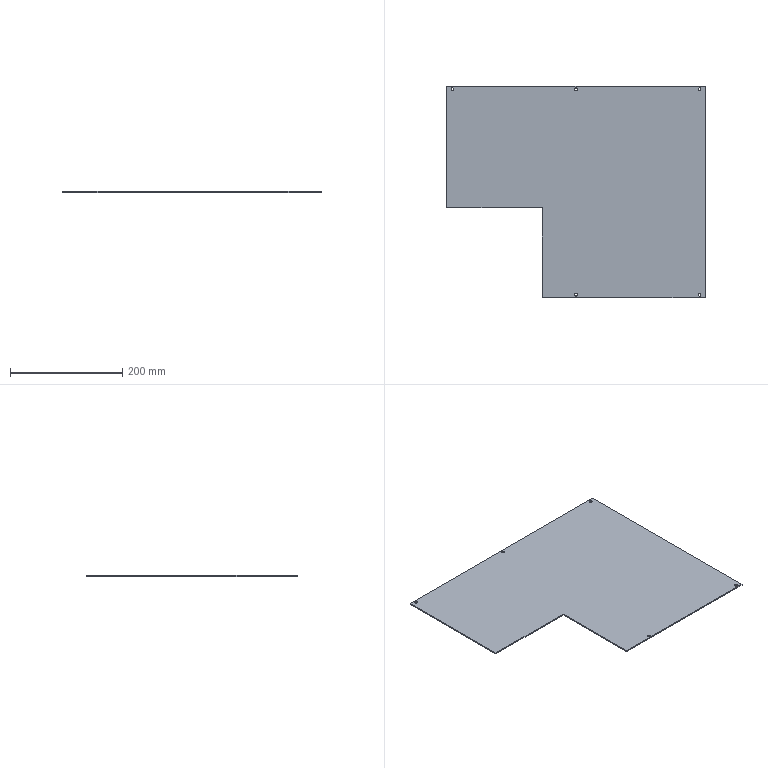Part | STEP file | Station three mount plate | 1 solid | 18 faces | box 460 x 376 x 2 mm | volume 291324 mm3 | cylinder 10 | plane 8 | commonest cylinder face diameters 5 x10
STEP:
#1=CARTESIAN_POINT('',(0.,0.,0.));
#2=DIRECTION('',(0.,0.,1.));
#3=DIRECTION('',(1.,0.,0.));
#4=AXIS2_PLACEMENT_3D('',#1,#2,#3);
#5=CARTESIAN_POINT('',(-217.5,183.,0.));
#6=VERTEX_POINT('',#5);
#7=CARTESIAN_POINT('',(-217.5,183.,2.));
#8=VERTEX_POINT('',#7);
#9=CARTESIAN_POINT('',(-217.5,183.,0.));
#10=DIRECTION('',(0.,0.,1.));
#11=VECTOR('',#10,1.);
#12=LINE('',#9,#11);
#13=CARTESIAN_POINT('',(-220.,183.,0.));
#14=DIRECTION('',(0.,0.,1.));
#15=DIRECTION('',(1.,0.,0.));
#16=AXIS2_PLACEMENT_3D('',#13,#14,#15);
#17=CYLINDRICAL_SURFACE('',#16,2.5);
#18=CARTESIAN_POINT('',(6.283,0.));
#19=DIRECTION('',(0.,1.));
#20=VECTOR('',#19,1.);
#21=LINE('',#18,#20);
#22=(GEOMETRIC_REPRESENTATION_CONTEXT(2)PARAMETRIC_REPRESENTATION_CONTEXT()REPRESENTATION_CONTEXT('',''));
#23=DEFINITIONAL_REPRESENTATION('',(#21),#22);
#24=PCURVE('',#17,#23);
#25=CARTESIAN_POINT('',(-220.,183.,0.));
#26=DIRECTION('',(0.,0.,1.));
#27=DIRECTION('',(1.,0.,0.));
#28=AXIS2_PLACEMENT_3D('',#25,#26,#27);
#29=CYLINDRICAL_SURFACE('',#28,2.5);
#30=CARTESIAN_POINT('',(0.,0.));
#31=DIRECTION('',(0.,1.));
#32=VECTOR('',#31,1.);
#33=LINE('',#30,#32);
#34=(GEOMETRIC_REPRESENTATION_CONTEXT(2)PARAMETRIC_REPRESENTATION_CONTEXT()REPRESENTATION_CONTEXT('',''));
#35=DEFINITIONAL_REPRESENTATION('',(#33),#34);
#36=PCURVE('',#29,#35);
#37=SURFACE_CURVE('',#12,(#24,#36),.PCURVE_S1.);
#38=EDGE_CURVE('',#6,#8,#37,.T.);
#39=ORIENTED_EDGE('',*,*,#38,.T.);
#40=CARTESIAN_POINT('',(-222.5,183.,2.));
#41=VERTEX_POINT('',#40);
#42=CARTESIAN_POINT('',(-220.,183.,2.));
#43=DIRECTION('',(0.,0.,-1.));
#44=DIRECTION('',(1.,0.,0.));
#45=AXIS2_PLACEMENT_3D('',#42,#43,#44);
#46=CIRCLE('',#45,2.5);
#47=CARTESIAN_POINT('',(6.283,2.));
#48=DIRECTION('',(-1.,0.));
#49=VECTOR('',#48,1.);
#50=LINE('',#47,#49);
#51=(GEOMETRIC_REPRESENTATION_CONTEXT(2)PARAMETRIC_REPRESENTATION_CONTEXT()REPRESENTATION_CONTEXT('',''));
#52=DEFINITIONAL_REPRESENTATION('',(#50),#51);
#53=PCURVE('',#17,#52);
#54=CARTESIAN_POINT('',(-230.,-188.,2.));
#55=DIRECTION('',(0.,0.,1.));
#56=DIRECTION('',(1.,0.,0.));
#57=AXIS2_PLACEMENT_3D('',#54,#55,#56);
#58=PLANE('',#57);
#59=CARTESIAN_POINT('',(12.5,371.));
#60=CARTESIAN_POINT('',(12.5,366.67));
#61=CARTESIAN_POINT('',(8.75,368.835));
#62=CARTESIAN_POINT('',(5.,371.));
#63=CARTESIAN_POINT('',(8.75,373.165));
#64=CARTESIAN_POINT('',(12.5,375.33));
#65=CARTESIAN_POINT('',(12.5,371.));
#66=(BOUNDED_CURVE()B_SPLINE_CURVE(2,(#59,#60,#61,#62,#63,#64,#65),.UNSPECIFIED.,.T.,.F.)B_SPLINE_CURVE_WITH_KNOTS((1,2,2,2,2,1),(-2.094,0.,2.094,4.189,6.283,8.378),.UNSPECIFIED.)CURVE()GEOMETRIC_REPRESENTATION_ITEM()RATIONAL_B_SPLINE_CURVE((1.,0.5,1.,0.5,1.,0.5,1.))REPRESENTATION_ITEM(''));
#67=(GEOMETRIC_REPRESENTATION_CONTEXT(2)PARAMETRIC_REPRESENTATION_CONTEXT()REPRESENTATION_CONTEXT('',''));
#68=DEFINITIONAL_REPRESENTATION('',(#66),#67);
#69=PCURVE('',#58,#68);
#70=SURFACE_CURVE('',#46,(#53,#69),.PCURVE_S1.);
#71=EDGE_CURVE('',#8,#41,#70,.T.);
#72=ORIENTED_EDGE('',*,*,#71,.T.);
#73=CARTESIAN_POINT('',(-222.5,183.,0.));
#74=VERTEX_POINT('',#73);
#75=CARTESIAN_POINT('',(-222.5,183.,0.));
#76=DIRECTION('',(0.,0.,1.));
#77=VECTOR('',#76,1.);
#78=LINE('',#75,#77);
#79=CARTESIAN_POINT('',(3.142,0.));
#80=DIRECTION('',(0.,1.));
#81=VECTOR('',#80,1.);
#82=LINE('',#79,#81);
#83=(GEOMETRIC_REPRESENTATION_CONTEXT(2)PARAMETRIC_REPRESENTATION_CONTEXT()REPRESENTATION_CONTEXT('',''));
#84=DEFINITIONAL_REPRESENTATION('',(#82),#83);
#85=PCURVE('',#17,#84);
#86=CARTESIAN_POINT('',(3.142,0.));
#87=DIRECTION('',(0.,1.));
#88=VECTOR('',#87,1.);
#89=LINE('',#86,#88);
#90=(GEOMETRIC_REPRESENTATION_CONTEXT(2)PARAMETRIC_REPRESENTATION_CONTEXT()REPRESENTATION_CONTEXT('',''));
#91=DEFINITIONAL_REPRESENTATION('',(#89),#90);
#92=PCURVE('',#29,#91);
#93=SURFACE_CURVE('',#78,(#85,#92),.PCURVE_S1.);
#94=EDGE_CURVE('',#74,#41,#93,.T.);
#95=ORIENTED_EDGE('',*,*,#94,.F.);
#96=CARTESIAN_POINT('',(-220.,183.,0.));
#97=DIRECTION('',(0.,0.,1.));
#98=DIRECTION('',(1.,0.,0.));
#99=AXIS2_PLACEMENT_3D('',#96,#97,#98);
#100=CIRCLE('',#99,2.5);
#101=CARTESIAN_POINT('',(0.,0.));
#102=DIRECTION('',(1.,0.));
#103=VECTOR('',#102,1.);
#104=LINE('',#101,#103);
#105=(GEOMETRIC_REPRESENTATION_CONTEXT(2)PARAMETRIC_REPRESENTATION_CONTEXT()REPRESENTATION_CONTEXT('',''));
#106=DEFINITIONAL_REPRESENTATION('',(#104),#105);
#107=PCURVE('',#17,#106);
#108=CARTESIAN_POINT('',(-230.,-188.,0.));
#109=DIRECTION('',(0.,0.,1.));
#110=DIRECTION('',(1.,0.,0.));
#111=AXIS2_PLACEMENT_3D('',#108,#109,#110);
#112=PLANE('',#111);
#113=CARTESIAN_POINT('',(10.,371.));
#114=DIRECTION('',(1.,0.));
#115=AXIS2_PLACEMENT_2D('',#113,#114);
#116=CIRCLE('',#115,2.5);
#117=(GEOMETRIC_REPRESENTATION_CONTEXT(2)PARAMETRIC_REPRESENTATION_CONTEXT()REPRESENTATION_CONTEXT('',''));
#118=DEFINITIONAL_REPRESENTATION('',(#116),#117);
#119=PCURVE('',#112,#118);
#120=SURFACE_CURVE('',#100,(#107,#119),.PCURVE_S1.);
#121=EDGE_CURVE('',#74,#6,#120,.T.);
#122=ORIENTED_EDGE('',*,*,#121,.T.);
#123=EDGE_LOOP('',(#39,#72,#95,#122));
#124=FACE_BOUND('',#123,.F.);
#125=ADVANCED_FACE('',(#124),#17,.F.);
#126=CARTESIAN_POINT('',(222.5,183.,0.));
#127=VERTEX_POINT('',#126);
#128=CARTESIAN_POINT('',(222.5,183.,2.));
#129=VERTEX_POINT('',#128);
#130=CARTESIAN_POINT('',(222.5,183.,0.));
#131=DIRECTION('',(0.,0.,1.));
#132=VECTOR('',#131,1.);
#133=LINE('',#130,#132);
#134=CARTESIAN_POINT('',(220.,183.,0.));
#135=DIRECTION('',(0.,0.,1.));
#136=DIRECTION('',(1.,0.,0.));
#137=AXIS2_PLACEMENT_3D('',#134,#135,#136);
#138=CYLINDRICAL_SURFACE('',#137,2.5);
#139=CARTESIAN_POINT('',(6.283,0.));
#140=DIRECTION('',(0.,1.));
#141=VECTOR('',#140,1.);
#142=LINE('',#139,#141);
#143=(GEOMETRIC_REPRESENTATION_CONTEXT(2)PARAMETRIC_REPRESENTATION_CONTEXT()REPRESENTATION_CONTEXT('',''));
#144=DEFINITIONAL_REPRESENTATION('',(#142),#143);
#145=PCURVE('',#138,#144);
#146=CARTESIAN_POINT('',(220.,183.,0.));
#147=DIRECTION('',(0.,0.,1.));
#148=DIRECTION('',(1.,0.,0.));
#149=AXIS2_PLACEMENT_3D('',#146,#147,#148);
#150=CYLINDRICAL_SURFACE('',#149,2.5);
#151=CARTESIAN_POINT('',(0.,0.));
#152=DIRECTION('',(0.,1.));
#153=VECTOR('',#152,1.);
#154=LINE('',#151,#153);
#155=(GEOMETRIC_REPRESENTATION_CONTEXT(2)PARAMETRIC_REPRESENTATION_CONTEXT()REPRESENTATION_CONTEXT('',''));
#156=DEFINITIONAL_REPRESENTATION('',(#154),#155);
#157=PCURVE('',#150,#156);
#158=SURFACE_CURVE('',#133,(#145,#157),.PCURVE_S1.);
#159=EDGE_CURVE('',#127,#129,#158,.T.);
#160=ORIENTED_EDGE('',*,*,#159,.T.);
#161=CARTESIAN_POINT('',(217.5,183.,2.));
#162=VERTEX_POINT('',#161);
#163=CARTESIAN_POINT('',(220.,183.,2.));
#164=DIRECTION('',(0.,0.,-1.));
#165=DIRECTION('',(1.,0.,0.));
#166=AXIS2_PLACEMENT_3D('',#163,#164,#165);
#167=CIRCLE('',#166,2.5);
#168=CARTESIAN_POINT('',(6.283,2.));
#169=DIRECTION('',(-1.,0.));
#170=VECTOR('',#169,1.);
#171=LINE('',#168,#170);
#172=(GEOMETRIC_REPRESENTATION_CONTEXT(2)PARAMETRIC_REPRESENTATION_CONTEXT()REPRESENTATION_CONTEXT('',''));
#173=DEFINITIONAL_REPRESENTATION('',(#171),#172);
#174=PCURVE('',#138,#173);
#175=CARTESIAN_POINT('',(452.5,371.));
#176=CARTESIAN_POINT('',(452.5,366.67));
#177=CARTESIAN_POINT('',(448.75,368.835));
#178=CARTESIAN_POINT('',(445.,371.));
#179=CARTESIAN_POINT('',(448.75,373.165));
#180=CARTESIAN_POINT('',(452.5,375.33));
#181=CARTESIAN_POINT('',(452.5,371.));
#182=(BOUNDED_CURVE()B_SPLINE_CURVE(2,(#175,#176,#177,#178,#179,#180,#181),.UNSPECIFIED.,.T.,.F.)B_SPLINE_CURVE_WITH_KNOTS((1,2,2,2,2,1),(-2.094,0.,2.094,4.189,6.283,8.378),.UNSPECIFIED.)CURVE()GEOMETRIC_REPRESENTATION_ITEM()RATIONAL_B_SPLINE_CURVE((1.,0.5,1.,0.5,1.,0.5,1.))REPRESENTATION_ITEM(''));
#183=(GEOMETRIC_REPRESENTATION_CONTEXT(2)PARAMETRIC_REPRESENTATION_CONTEXT()REPRESENTATION_CONTEXT('',''));
#184=DEFINITIONAL_REPRESENTATION('',(#182),#183);
#185=PCURVE('',#58,#184);
#186=SURFACE_CURVE('',#167,(#174,#185),.PCURVE_S1.);
#187=EDGE_CURVE('',#129,#162,#186,.T.);
#188=ORIENTED_EDGE('',*,*,#187,.T.);
#189=CARTESIAN_POINT('',(217.5,183.,0.));
#190=VERTEX_POINT('',#189);
#191=CARTESIAN_POINT('',(217.5,183.,0.));
#192=DIRECTION('',(0.,0.,1.));
#193=VECTOR('',#192,1.);
#194=LINE('',#191,#193);
#195=CARTESIAN_POINT('',(3.142,0.));
#196=DIRECTION('',(0.,1.));
#197=VECTOR('',#196,1.);
#198=LINE('',#195,#197);
#199=(GEOMETRIC_REPRESENTATION_CONTEXT(2)PARAMETRIC_REPRESENTATION_CONTEXT()REPRESENTATION_CONTEXT('',''));
#200=DEFINITIONAL_REPRESENTATION('',(#198),#199);
#201=PCURVE('',#138,#200);
#202=CARTESIAN_POINT('',(3.142,0.));
#203=DIRECTION('',(0.,1.));
#204=VECTOR('',#203,1.);
#205=LINE('',#202,#204);
#206=(GEOMETRIC_REPRESENTATION_CONTEXT(2)PARAMETRIC_REPRESENTATION_CONTEXT()REPRESENTATION_CONTEXT('',''));
#207=DEFINITIONAL_REPRESENTATION('',(#205),#206);
#208=PCURVE('',#150,#207);
#209=SURFACE_CURVE('',#194,(#201,#208),.PCURVE_S1.);
#210=EDGE_CURVE('',#190,#162,#209,.T.);
#211=ORIENTED_EDGE('',*,*,#210,.F.);
#212=CARTESIAN_POINT('',(220.,183.,0.));
#213=DIRECTION('',(0.,0.,1.));
#214=DIRECTION('',(1.,0.,0.));
#215=AXIS2_PLACEMENT_3D('',#212,#213,#214);
#216=CIRCLE('',#215,2.5);
#217=CARTESIAN_POINT('',(0.,0.));
#218=DIRECTION('',(1.,0.));
#219=VECTOR('',#218,1.);
#220=LINE('',#217,#219);
#221=(GEOMETRIC_REPRESENTATION_CONTEXT(2)PARAMETRIC_REPRESENTATION_CONTEXT()REPRESENTATION_CONTEXT('',''));
#222=DEFINITIONAL_REPRESENTATION('',(#220),#221);
#223=PCURVE('',#138,#222);
#224=CARTESIAN_POINT('',(450.,371.));
#225=DIRECTION('',(1.,0.));
#226=AXIS2_PLACEMENT_2D('',#224,#225);
#227=CIRCLE('',#226,2.5);
#228=(GEOMETRIC_REPRESENTATION_CONTEXT(2)PARAMETRIC_REPRESENTATION_CONTEXT()REPRESENTATION_CONTEXT('',''));
#229=DEFINITIONAL_REPRESENTATION('',(#227),#228);
#230=PCURVE('',#112,#229);
#231=SURFACE_CURVE('',#216,(#223,#230),.PCURVE_S1.);
#232=EDGE_CURVE('',#190,#127,#231,.T.);
#233=ORIENTED_EDGE('',*,*,#232,.T.);
#234=EDGE_LOOP('',(#160,#188,#211,#233));
#235=FACE_BOUND('',#234,.F.);
#236=ADVANCED_FACE('',(#235),#138,.F.);
#237=CARTESIAN_POINT('',(2.5,-183.,0.));
#238=VERTEX_POINT('',#237);
#239=CARTESIAN_POINT('',(2.5,-183.,2.));
#240=VERTEX_POINT('',#239);
#241=CARTESIAN_POINT('',(2.5,-183.,0.));
#242=DIRECTION('',(0.,0.,1.));
#243=VECTOR('',#242,1.);
#244=LINE('',#241,#243);
#245=CARTESIAN_POINT('',(0.,-183.,0.));
#246=DIRECTION('',(0.,0.,1.));
#247=DIRECTION('',(1.,0.,0.));
#248=AXIS2_PLACEMENT_3D('',#245,#246,#247);
#249=CYLINDRICAL_SURFACE('',#248,2.5);
#250=CARTESIAN_POINT('',(6.283,0.));
#251=DIRECTION('',(0.,1.));
#252=VECTOR('',#251,1.);
#253=LINE('',#250,#252);
#254=(GEOMETRIC_REPRESENTATION_CONTEXT(2)PARAMETRIC_REPRESENTATION_CONTEXT()REPRESENTATION_CONTEXT('',''));
#255=DEFINITIONAL_REPRESENTATION('',(#253),#254);
#256=PCURVE('',#249,#255);
#257=CARTESIAN_POINT('',(0.,-183.,0.));
#258=DIRECTION('',(0.,0.,1.));
#259=DIRECTION('',(1.,0.,0.));
#260=AXIS2_PLACEMENT_3D('',#257,#258,#259);
#261=CYLINDRICAL_SURFACE('',#260,2.5);
#262=CARTESIAN_POINT('',(0.,0.));
#263=DIRECTION('',(0.,1.));
#264=VECTOR('',#263,1.);
#265=LINE('',#262,#264);
#266=(GEOMETRIC_REPRESENTATION_CONTEXT(2)PARAMETRIC_REPRESENTATION_CONTEXT()REPRESENTATION_CONTEXT('',''));
#267=DEFINITIONAL_REPRESENTATION('',(#265),#266);
#268=PCURVE('',#261,#267);
#269=SURFACE_CURVE('',#244,(#256,#268),.PCURVE_S1.);
#270=EDGE_CURVE('',#238,#240,#269,.T.);
#271=ORIENTED_EDGE('',*,*,#270,.T.);
#272=CARTESIAN_POINT('',(-2.5,-183.,2.));
#273=VERTEX_POINT('',#272);
#274=CARTESIAN_POINT('',(0.,-183.,2.));
#275=DIRECTION('',(0.,0.,-1.));
#276=DIRECTION('',(1.,0.,0.));
#277=AXIS2_PLACEMENT_3D('',#274,#275,#276);
#278=CIRCLE('',#277,2.5);
#279=CARTESIAN_POINT('',(6.283,2.));
#280=DIRECTION('',(-1.,0.));
#281=VECTOR('',#280,1.);
#282=LINE('',#279,#281);
#283=(GEOMETRIC_REPRESENTATION_CONTEXT(2)PARAMETRIC_REPRESENTATION_CONTEXT()REPRESENTATION_CONTEXT('',''));
#284=DEFINITIONAL_REPRESENTATION('',(#282),#283);
#285=PCURVE('',#249,#284);
#286=CARTESIAN_POINT('',(232.5,5.));
#287=CARTESIAN_POINT('',(232.5,0.6699));
#288=CARTESIAN_POINT('',(228.75,2.835));
#289=CARTESIAN_POINT('',(225.,5.));
#290=CARTESIAN_POINT('',(228.75,7.165));
#291=CARTESIAN_POINT('',(232.5,9.33));
#292=CARTESIAN_POINT('',(232.5,5.));
#293=(BOUNDED_CURVE()B_SPLINE_CURVE(2,(#286,#287,#288,#289,#290,#291,#292),.UNSPECIFIED.,.T.,.F.)B_SPLINE_CURVE_WITH_KNOTS((1,2,2,2,2,1),(-2.094,0.,2.094,4.189,6.283,8.378),.UNSPECIFIED.)CURVE()GEOMETRIC_REPRESENTATION_ITEM()RATIONAL_B_SPLINE_CURVE((1.,0.5,1.,0.5,1.,0.5,1.))REPRESENTATION_ITEM(''));
#294=(GEOMETRIC_REPRESENTATION_CONTEXT(2)PARAMETRIC_REPRESENTATION_CONTEXT()REPRESENTATION_CONTEXT('',''));
#295=DEFINITIONAL_REPRESENTATION('',(#293),#294);
#296=PCURVE('',#58,#295);
#297=SURFACE_CURVE('',#278,(#285,#296),.PCURVE_S1.);
#298=EDGE_CURVE('',#240,#273,#297,.T.);
#299=ORIENTED_EDGE('',*,*,#298,.T.);
#300=CARTESIAN_POINT('',(-2.5,-183.,0.));
#301=VERTEX_POINT('',#300);
#302=CARTESIAN_POINT('',(-2.5,-183.,0.));
#303=DIRECTION('',(0.,0.,1.));
#304=VECTOR('',#303,1.);
#305=LINE('',#302,#304);
#306=CARTESIAN_POINT('',(3.142,0.));
#307=DIRECTION('',(0.,1.));
#308=VECTOR('',#307,1.);
#309=LINE('',#306,#308);
#310=(GEOMETRIC_REPRESENTATION_CONTEXT(2)PARAMETRIC_REPRESENTATION_CONTEXT()REPRESENTATION_CONTEXT('',''));
#311=DEFINITIONAL_REPRESENTATION('',(#309),#310);
#312=PCURVE('',#249,#311);
#313=CARTESIAN_POINT('',(3.142,0.));
#314=DIRECTION('',(0.,1.));
#315=VECTOR('',#314,1.);
#316=LINE('',#313,#315);
#317=(GEOMETRIC_REPRESENTATION_CONTEXT(2)PARAMETRIC_REPRESENTATION_CONTEXT()REPRESENTATION_CONTEXT('',''));
#318=DEFINITIONAL_REPRESENTATION('',(#316),#317);
#319=PCURVE('',#261,#318);
#320=SURFACE_CURVE('',#305,(#312,#319),.PCURVE_S1.);
#321=EDGE_CURVE('',#301,#273,#320,.T.);
#322=ORIENTED_EDGE('',*,*,#321,.F.);
#323=CARTESIAN_POINT('',(0.,-183.,0.));
#324=DIRECTION('',(0.,0.,1.));
#325=DIRECTION('',(1.,0.,0.));
#326=AXIS2_PLACEMENT_3D('',#323,#324,#325);
#327=CIRCLE('',#326,2.5);
#328=CARTESIAN_POINT('',(0.,0.));
#329=DIRECTION('',(1.,0.));
#330=VECTOR('',#329,1.);
#331=LINE('',#328,#330);
#332=(GEOMETRIC_REPRESENTATION_CONTEXT(2)PARAMETRIC_REPRESENTATION_CONTEXT()REPRESENTATION_CONTEXT('',''));
#333=DEFINITIONAL_REPRESENTATION('',(#331),#332);
#334=PCURVE('',#249,#333);
#335=CARTESIAN_POINT('',(230.,5.));
#336=DIRECTION('',(1.,0.));
#337=AXIS2_PLACEMENT_2D('',#335,#336);
#338=CIRCLE('',#337,2.5);
#339=(GEOMETRIC_REPRESENTATION_CONTEXT(2)PARAMETRIC_REPRESENTATION_CONTEXT()REPRESENTATION_CONTEXT('',''));
#340=DEFINITIONAL_REPRESENTATION('',(#338),#339);
#341=PCURVE('',#112,#340);
#342=SURFACE_CURVE('',#327,(#334,#341),.PCURVE_S1.);
#343=EDGE_CURVE('',#301,#238,#342,.T.);
#344=ORIENTED_EDGE('',*,*,#343,.T.);
#345=EDGE_LOOP('',(#271,#299,#322,#344));
#346=FACE_BOUND('',#345,.F.);
#347=ADVANCED_FACE('',(#346),#249,.F.);
#348=CARTESIAN_POINT('',(222.5,-183.,0.));
#349=VERTEX_POINT('',#348);
#350=CARTESIAN_POINT('',(222.5,-183.,2.));
#351=VERTEX_POINT('',#350);
#352=CARTESIAN_POINT('',(222.5,-183.,0.));
#353=DIRECTION('',(0.,0.,1.));
#354=VECTOR('',#353,1.);
#355=LINE('',#352,#354);
#356=CARTESIAN_POINT('',(220.,-183.,0.));
#357=DIRECTION('',(0.,0.,1.));
#358=DIRECTION('',(1.,0.,0.));
#359=AXIS2_PLACEMENT_3D('',#356,#357,#358);
#360=CYLINDRICAL_SURFACE('',#359,2.5);
#361=CARTESIAN_POINT('',(6.283,0.));
#362=DIRECTION('',(0.,1.));
#363=VECTOR('',#362,1.);
#364=LINE('',#361,#363);
#365=(GEOMETRIC_REPRESENTATION_CONTEXT(2)PARAMETRIC_REPRESENTATION_CONTEXT()REPRESENTATION_CONTEXT('',''));
#366=DEFINITIONAL_REPRESENTATION('',(#364),#365);
#367=PCURVE('',#360,#366);
#368=CARTESIAN_POINT('',(220.,-183.,0.));
#369=DIRECTION('',(0.,0.,1.));
#370=DIRECTION('',(1.,0.,0.));
#371=AXIS2_PLACEMENT_3D('',#368,#369,#370);
#372=CYLINDRICAL_SURFACE('',#371,2.5);
#373=CARTESIAN_POINT('',(0.,0.));
#374=DIRECTION('',(0.,1.));
#375=VECTOR('',#374,1.);
#376=LINE('',#373,#375);
#377=(GEOMETRIC_REPRESENTATION_CONTEXT(2)PARAMETRIC_REPRESENTATION_CONTEXT()REPRESENTATION_CONTEXT('',''));
#378=DEFINITIONAL_REPRESENTATION('',(#376),#377);
#379=PCURVE('',#372,#378);
#380=SURFACE_CURVE('',#355,(#367,#379),.PCURVE_S1.);
#381=EDGE_CURVE('',#349,#351,#380,.T.);
#382=ORIENTED_EDGE('',*,*,#381,.T.);
#383=CARTESIAN_POINT('',(217.5,-183.,2.));
#384=VERTEX_POINT('',#383);
#385=CARTESIAN_POINT('',(220.,-183.,2.));
#386=DIRECTION('',(0.,0.,-1.));
#387=DIRECTION('',(1.,0.,0.));
#388=AXIS2_PLACEMENT_3D('',#385,#386,#387);
#389=CIRCLE('',#388,2.5);
#390=CARTESIAN_POINT('',(6.283,2.));
#391=DIRECTION('',(-1.,0.));
#392=VECTOR('',#391,1.);
#393=LINE('',#390,#392);
#394=(GEOMETRIC_REPRESENTATION_CONTEXT(2)PARAMETRIC_REPRESENTATION_CONTEXT()REPRESENTATION_CONTEXT('',''));
#395=DEFINITIONAL_REPRESENTATION('',(#393),#394);
#396=PCURVE('',#360,#395);
#397=CARTESIAN_POINT('',(452.5,5.));
#398=CARTESIAN_POINT('',(452.5,0.6699));
#399=CARTESIAN_POINT('',(448.75,2.835));
#400=CARTESIAN_POINT('',(445.,5.));
#401=CARTESIAN_POINT('',(448.75,7.165));
#402=CARTESIAN_POINT('',(452.5,9.33));
#403=CARTESIAN_POINT('',(452.5,5.));
#404=(BOUNDED_CURVE()B_SPLINE_CURVE(2,(#397,#398,#399,#400,#401,#402,#403),.UNSPECIFIED.,.T.,.F.)B_SPLINE_CURVE_WITH_KNOTS((1,2,2,2,2,1),(-2.094,0.,2.094,4.189,6.283,8.378),.UNSPECIFIED.)CURVE()GEOMETRIC_REPRESENTATION_ITEM()RATIONAL_B_SPLINE_CURVE((1.,0.5,1.,0.5,1.,0.5,1.))REPRESENTATION_ITEM(''));
#405=(GEOMETRIC_REPRESENTATION_CONTEXT(2)PARAMETRIC_REPRESENTATION_CONTEXT()REPRESENTATION_CONTEXT('',''));
#406=DEFINITIONAL_REPRESENTATION('',(#404),#405);
#407=PCURVE('',#58,#406);
#408=SURFACE_CURVE('',#389,(#396,#407),.PCURVE_S1.);
#409=EDGE_CURVE('',#351,#384,#408,.T.);
#410=ORIENTED_EDGE('',*,*,#409,.T.);
#411=CARTESIAN_POINT('',(217.5,-183.,0.));
#412=VERTEX_POINT('',#411);
#413=CARTESIAN_POINT('',(217.5,-183.,0.));
#414=DIRECTION('',(0.,0.,1.));
#415=VECTOR('',#414,1.);
#416=LINE('',#413,#415);
#417=CARTESIAN_POINT('',(3.142,0.));
#418=DIRECTION('',(0.,1.));
#419=VECTOR('',#418,1.);
#420=LINE('',#417,#419);
#421=(GEOMETRIC_REPRESENTATION_CONTEXT(2)PARAMETRIC_REPRESENTATION_CONTEXT()REPRESENTATION_CONTEXT('',''));
#422=DEFINITIONAL_REPRESENTATION('',(#420),#421);
#423=PCURVE('',#360,#422);
#424=CARTESIAN_POINT('',(3.142,0.));
#425=DIRECTION('',(0.,1.));
#426=VECTOR('',#425,1.);
#427=LINE('',#424,#426);
#428=(GEOMETRIC_REPRESENTATION_CONTEXT(2)PARAMETRIC_REPRESENTATION_CONTEXT()REPRESENTATION_CONTEXT('',''));
#429=DEFINITIONAL_REPRESENTATION('',(#427),#428);
#430=PCURVE('',#372,#429);
#431=SURFACE_CURVE('',#416,(#423,#430),.PCURVE_S1.);
#432=EDGE_CURVE('',#412,#384,#431,.T.);
#433=ORIENTED_EDGE('',*,*,#432,.F.);
#434=CARTESIAN_POINT('',(220.,-183.,0.));
#435=DIRECTION('',(0.,0.,1.));
#436=DIRECTION('',(1.,0.,0.));
#437=AXIS2_PLACEMENT_3D('',#434,#435,#436);
#438=CIRCLE('',#437,2.5);
#439=CARTESIAN_POINT('',(0.,0.));
#440=DIRECTION('',(1.,0.));
#441=VECTOR('',#440,1.);
#442=LINE('',#439,#441);
#443=(GEOMETRIC_REPRESENTATION_CONTEXT(2)PARAMETRIC_REPRESENTATION_CONTEXT()REPRESENTATION_CONTEXT('',''));
#444=DEFINITIONAL_REPRESENTATION('',(#442),#443);
#445=PCURVE('',#360,#444);
#446=CARTESIAN_POINT('',(450.,5.));
#447=DIRECTION('',(1.,0.));
#448=AXIS2_PLACEMENT_2D('',#446,#447);
#449=CIRCLE('',#448,2.5);
#450=(GEOMETRIC_REPRESENTATION_CONTEXT(2)PARAMETRIC_REPRESENTATION_CONTEXT()REPRESENTATION_CONTEXT('',''));
#451=DEFINITIONAL_REPRESENTATION('',(#449),#450);
#452=PCURVE('',#112,#451);
#453=SURFACE_CURVE('',#438,(#445,#452),.PCURVE_S1.);
#454=EDGE_CURVE('',#412,#349,#453,.T.);
#455=ORIENTED_EDGE('',*,*,#454,.T.);
#456=EDGE_LOOP('',(#382,#410,#433,#455));
#457=FACE_BOUND('',#456,.F.);
#458=ADVANCED_FACE('',(#457),#360,.F.);
#459=CARTESIAN_POINT('',(2.5,183.,0.));
#460=VERTEX_POINT('',#459);
#461=CARTESIAN_POINT('',(2.5,183.,2.));
#462=VERTEX_POINT('',#461);
#463=CARTESIAN_POINT('',(2.5,183.,0.));
#464=DIRECTION('',(0.,0.,1.));
#465=VECTOR('',#464,1.);
#466=LINE('',#463,#465);
#467=CARTESIAN_POINT('',(0.,183.,0.));
#468=DIRECTION('',(0.,0.,1.));
#469=DIRECTION('',(1.,0.,0.));
#470=AXIS2_PLACEMENT_3D('',#467,#468,#469);
#471=CYLINDRICAL_SURFACE('',#470,2.5);
#472=CARTESIAN_POINT('',(6.283,0.));
#473=DIRECTION('',(0.,1.));
#474=VECTOR('',#473,1.);
#475=LINE('',#472,#474);
#476=(GEOMETRIC_REPRESENTATION_CONTEXT(2)PARAMETRIC_REPRESENTATION_CONTEXT()REPRESENTATION_CONTEXT('',''));
#477=DEFINITIONAL_REPRESENTATION('',(#475),#476);
#478=PCURVE('',#471,#477);
#479=CARTESIAN_POINT('',(0.,183.,0.));
#480=DIRECTION('',(0.,0.,1.));
#481=DIRECTION('',(1.,0.,0.));
#482=AXIS2_PLACEMENT_3D('',#479,#480,#481);
#483=CYLINDRICAL_SURFACE('',#482,2.5);
#484=CARTESIAN_POINT('',(0.,0.));
#485=DIRECTION('',(0.,1.));
#486=VECTOR('',#485,1.);
#487=LINE('',#484,#486);
#488=(GEOMETRIC_REPRESENTATION_CONTEXT(2)PARAMETRIC_REPRESENTATION_CONTEXT()REPRESENTATION_CONTEXT('',''));
#489=DEFINITIONAL_REPRESENTATION('',(#487),#488);
#490=PCURVE('',#483,#489);
#491=SURFACE_CURVE('',#466,(#478,#490),.PCURVE_S1.);
#492=EDGE_CURVE('',#460,#462,#491,.T.);
#493=ORIENTED_EDGE('',*,*,#492,.T.);
#494=CARTESIAN_POINT('',(-2.5,183.,2.));
#495=VERTEX_POINT('',#494);
#496=CARTESIAN_POINT('',(0.,183.,2.));
#497=DIRECTION('',(0.,0.,-1.));
#498=DIRECTION('',(1.,0.,0.));
#499=AXIS2_PLACEMENT_3D('',#496,#497,#498);
#500=CIRCLE('',#499,2.5);
#501=CARTESIAN_POINT('',(6.283,2.));
#502=DIRECTION('',(-1.,0.));
#503=VECTOR('',#502,1.);
#504=LINE('',#501,#503);
#505=(GEOMETRIC_REPRESENTATION_CONTEXT(2)PARAMETRIC_REPRESENTATION_CONTEXT()REPRESENTATION_CONTEXT('',''));
#506=DEFINITIONAL_REPRESENTATION('',(#504),#505);
#507=PCURVE('',#471,#506);
#508=CARTESIAN_POINT('',(232.5,371.));
#509=CARTESIAN_POINT('',(232.5,366.67));
#510=CARTESIAN_POINT('',(228.75,368.835));
#511=CARTESIAN_POINT('',(225.,371.));
#512=CARTESIAN_POINT('',(228.75,373.165));
#513=CARTESIAN_POINT('',(232.5,375.33));
#514=CARTESIAN_POINT('',(232.5,371.));
#515=(BOUNDED_CURVE()B_SPLINE_CURVE(2,(#508,#509,#510,#511,#512,#513,#514),.UNSPECIFIED.,.T.,.F.)B_SPLINE_CURVE_WITH_KNOTS((1,2,2,2,2,1),(-2.094,0.,2.094,4.189,6.283,8.378),.UNSPECIFIED.)CURVE()GEOMETRIC_REPRESENTATION_ITEM()RATIONAL_B_SPLINE_CURVE((1.,0.5,1.,0.5,1.,0.5,1.))REPRESENTATION_ITEM(''));
#516=(GEOMETRIC_REPRESENTATION_CONTEXT(2)PARAMETRIC_REPRESENTATION_CONTEXT()REPRESENTATION_CONTEXT('',''));
#517=DEFINITIONAL_REPRESENTATION('',(#515),#516);
#518=PCURVE('',#58,#517);
#519=SURFACE_CURVE('',#500,(#507,#518),.PCURVE_S1.);
#520=EDGE_CURVE('',#462,#495,#519,.T.);
#521=ORIENTED_EDGE('',*,*,#520,.T.);
#522=CARTESIAN_POINT('',(-2.5,183.,0.));
#523=VERTEX_POINT('',#522);
#524=CARTESIAN_POINT('',(-2.5,183.,0.));
#525=DIRECTION('',(0.,0.,1.));
#526=VECTOR('',#525,1.);
#527=LINE('',#524,#526);
#528=CARTESIAN_POINT('',(3.142,0.));
#529=DIRECTION('',(0.,1.));
#530=VECTOR('',#529,1.);
#531=LINE('',#528,#530);
#532=(GEOMETRIC_REPRESENTATION_CONTEXT(2)PARAMETRIC_REPRESENTATION_CONTEXT()REPRESENTATION_CONTEXT('',''));
#533=DEFINITIONAL_REPRESENTATION('',(#531),#532);
#534=PCURVE('',#471,#533);
#535=CARTESIAN_POINT('',(3.142,0.));
#536=DIRECTION('',(0.,1.));
#537=VECTOR('',#536,1.);
#538=LINE('',#535,#537);
#539=(GEOMETRIC_REPRESENTATION_CONTEXT(2)PARAMETRIC_REPRESENTATION_CONTEXT()REPRESENTATION_CONTEXT('',''));
#540=DEFINITIONAL_REPRESENTATION('',(#538),#539);
#541=PCURVE('',#483,#540);
#542=SURFACE_CURVE('',#527,(#534,#541),.PCURVE_S1.);
#543=EDGE_CURVE('',#523,#495,#542,.T.);
#544=ORIENTED_EDGE('',*,*,#543,.F.);
#545=CARTESIAN_POINT('',(0.,183.,0.));
#546=DIRECTION('',(0.,0.,1.));
#547=DIRECTION('',(1.,0.,0.));
#548=AXIS2_PLACEMENT_3D('',#545,#546,#547);
#549=CIRCLE('',#548,2.5);
#550=CARTESIAN_POINT('',(0.,0.));
#551=DIRECTION('',(1.,0.));
#552=VECTOR('',#551,1.);
#553=LINE('',#550,#552);
#554=(GEOMETRIC_REPRESENTATION_CONTEXT(2)PARAMETRIC_REPRESENTATION_CONTEXT()REPRESENTATION_CONTEXT('',''));
#555=DEFINITIONAL_REPRESENTATION('',(#553),#554);
#556=PCURVE('',#471,#555);
#557=CARTESIAN_POINT('',(230.,371.));
#558=DIRECTION('',(1.,0.));
#559=AXIS2_PLACEMENT_2D('',#557,#558);
#560=CIRCLE('',#559,2.5);
#561=(GEOMETRIC_REPRESENTATION_CONTEXT(2)PARAMETRIC_REPRESENTATION_CONTEXT()REPRESENTATION_CONTEXT('',''));
#562=DEFINITIONAL_REPRESENTATION('',(#560),#561);
#563=PCURVE('',#112,#562);
#564=SURFACE_CURVE('',#549,(#556,#563),.PCURVE_S1.);
#565=EDGE_CURVE('',#523,#460,#564,.T.);
#566=ORIENTED_EDGE('',*,*,#565,.T.);
#567=EDGE_LOOP('',(#493,#521,#544,#566));
#568=FACE_BOUND('',#567,.F.);
#569=ADVANCED_FACE('',(#568),#471,.F.);
#570=ORIENTED_EDGE('',*,*,#71,.T.);
#571=CARTESIAN_POINT('',(-220.,183.,2.));
#572=DIRECTION('',(0.,0.,-1.));
#573=DIRECTION('',(1.,0.,0.));
#574=AXIS2_PLACEMENT_3D('',#571,#572,#573);
#575=CIRCLE('',#574,2.5);
#576=CARTESIAN_POINT('',(12.5,371.));
#577=CARTESIAN_POINT('',(12.5,366.67));
#578=CARTESIAN_POINT('',(8.75,368.835));
#579=CARTESIAN_POINT('',(5.,371.));
#580=CARTESIAN_POINT('',(8.75,373.165));
#581=CARTESIAN_POINT('',(12.5,375.33));
#582=CARTESIAN_POINT('',(12.5,371.));
#583=(BOUNDED_CURVE()B_SPLINE_CURVE(2,(#576,#577,#578,#579,#580,#581,#582),.UNSPECIFIED.,.T.,.F.)B_SPLINE_CURVE_WITH_KNOTS((1,2,2,2,2,1),(-2.094,0.,2.094,4.189,6.283,8.378),.UNSPECIFIED.)CURVE()GEOMETRIC_REPRESENTATION_ITEM()RATIONAL_B_SPLINE_CURVE((1.,0.5,1.,0.5,1.,0.5,1.))REPRESENTATION_ITEM(''));
#584=(GEOMETRIC_REPRESENTATION_CONTEXT(2)PARAMETRIC_REPRESENTATION_CONTEXT()REPRESENTATION_CONTEXT('',''));
#585=DEFINITIONAL_REPRESENTATION('',(#583),#584);
#586=PCURVE('',#58,#585);
#587=CARTESIAN_POINT('',(6.283,2.));
#588=DIRECTION('',(-1.,0.));
#589=VECTOR('',#588,1.);
#590=LINE('',#587,#589);
#591=(GEOMETRIC_REPRESENTATION_CONTEXT(2)PARAMETRIC_REPRESENTATION_CONTEXT()REPRESENTATION_CONTEXT('',''));
#592=DEFINITIONAL_REPRESENTATION('',(#590),#591);
#593=PCURVE('',#29,#592);
#594=SURFACE_CURVE('',#575,(#586,#593),.PCURVE_S1.);
#595=EDGE_CURVE('',#41,#8,#594,.T.);
#596=ORIENTED_EDGE('',*,*,#595,.T.);
#597=EDGE_LOOP('',(#570,#596));
#598=FACE_BOUND('',#597,.T.);
#599=ORIENTED_EDGE('',*,*,#187,.T.);
#600=CARTESIAN_POINT('',(220.,183.,2.));
#601=DIRECTION('',(0.,0.,-1.));
#602=DIRECTION('',(1.,0.,0.));
#603=AXIS2_PLACEMENT_3D('',#600,#601,#602);
#604=CIRCLE('',#603,2.5);
#605=CARTESIAN_POINT('',(452.5,371.));
#606=CARTESIAN_POINT('',(452.5,366.67));
#607=CARTESIAN_POINT('',(448.75,368.835));
#608=CARTESIAN_POINT('',(445.,371.));
#609=CARTESIAN_POINT('',(448.75,373.165));
#610=CARTESIAN_POINT('',(452.5,375.33));
#611=CARTESIAN_POINT('',(452.5,371.));
#612=(BOUNDED_CURVE()B_SPLINE_CURVE(2,(#605,#606,#607,#608,#609,#610,#611),.UNSPECIFIED.,.T.,.F.)B_SPLINE_CURVE_WITH_KNOTS((1,2,2,2,2,1),(-2.094,0.,2.094,4.189,6.283,8.378),.UNSPECIFIED.)CURVE()GEOMETRIC_REPRESENTATION_ITEM()RATIONAL_B_SPLINE_CURVE((1.,0.5,1.,0.5,1.,0.5,1.))REPRESENTATION_ITEM(''));
#613=(GEOMETRIC_REPRESENTATION_CONTEXT(2)PARAMETRIC_REPRESENTATION_CONTEXT()REPRESENTATION_CONTEXT('',''));
#614=DEFINITIONAL_REPRESENTATION('',(#612),#613);
#615=PCURVE('',#58,#614);
#616=CARTESIAN_POINT('',(6.283,2.));
#617=DIRECTION('',(-1.,0.));
#618=VECTOR('',#617,1.);
#619=LINE('',#616,#618);
#620=(GEOMETRIC_REPRESENTATION_CONTEXT(2)PARAMETRIC_REPRESENTATION_CONTEXT()REPRESENTATION_CONTEXT('',''));
#621=DEFINITIONAL_REPRESENTATION('',(#619),#620);
#622=PCURVE('',#150,#621);
#623=SURFACE_CURVE('',#604,(#615,#622),.PCURVE_S1.);
#624=EDGE_CURVE('',#162,#129,#623,.T.);
#625=ORIENTED_EDGE('',*,*,#624,.T.);
#626=EDGE_LOOP('',(#599,#625));
#627=FACE_BOUND('',#626,.T.);
#628=ORIENTED_EDGE('',*,*,#298,.T.);
#629=CARTESIAN_POINT('',(0.,-183.,2.));
#630=DIRECTION('',(0.,0.,-1.));
#631=DIRECTION('',(1.,0.,0.));
#632=AXIS2_PLACEMENT_3D('',#629,#630,#631);
#633=CIRCLE('',#632,2.5);
#634=CARTESIAN_POINT('',(232.5,5.));
#635=CARTESIAN_POINT('',(232.5,0.6699));
#636=CARTESIAN_POINT('',(228.75,2.835));
#637=CARTESIAN_POINT('',(225.,5.));
#638=CARTESIAN_POINT('',(228.75,7.165));
#639=CARTESIAN_POINT('',(232.5,9.33));
#640=CARTESIAN_POINT('',(232.5,5.));
#641=(BOUNDED_CURVE()B_SPLINE_CURVE(2,(#634,#635,#636,#637,#638,#639,#640),.UNSPECIFIED.,.T.,.F.)B_SPLINE_CURVE_WITH_KNOTS((1,2,2,2,2,1),(-2.094,0.,2.094,4.189,6.283,8.378),.UNSPECIFIED.)CURVE()GEOMETRIC_REPRESENTATION_ITEM()RATIONAL_B_SPLINE_CURVE((1.,0.5,1.,0.5,1.,0.5,1.))REPRESENTATION_ITEM(''));
#642=(GEOMETRIC_REPRESENTATION_CONTEXT(2)PARAMETRIC_REPRESENTATION_CONTEXT()REPRESENTATION_CONTEXT('',''));
#643=DEFINITIONAL_REPRESENTATION('',(#641),#642);
#644=PCURVE('',#58,#643);
#645=CARTESIAN_POINT('',(6.283,2.));
#646=DIRECTION('',(-1.,0.));
#647=VECTOR('',#646,1.);
#648=LINE('',#645,#647);
#649=(GEOMETRIC_REPRESENTATION_CONTEXT(2)PARAMETRIC_REPRESENTATION_CONTEXT()REPRESENTATION_CONTEXT('',''));
#650=DEFINITIONAL_REPRESENTATION('',(#648),#649);
#651=PCURVE('',#261,#650);
#652=SURFACE_CURVE('',#633,(#644,#651),.PCURVE_S1.);
#653=EDGE_CURVE('',#273,#240,#652,.T.);
#654=ORIENTED_EDGE('',*,*,#653,.T.);
#655=EDGE_LOOP('',(#628,#654));
#656=FACE_BOUND('',#655,.T.);
#657=ORIENTED_EDGE('',*,*,#409,.T.);
#658=CARTESIAN_POINT('',(220.,-183.,2.));
#659=DIRECTION('',(0.,0.,-1.));
#660=DIRECTION('',(1.,0.,0.));
#661=AXIS2_PLACEMENT_3D('',#658,#659,#660);
#662=CIRCLE('',#661,2.5);
#663=CARTESIAN_POINT('',(452.5,5.));
#664=CARTESIAN_POINT('',(452.5,0.6699));
#665=CARTESIAN_POINT('',(448.75,2.835));
#666=CARTESIAN_POINT('',(445.,5.));
#667=CARTESIAN_POINT('',(448.75,7.165));
#668=CARTESIAN_POINT('',(452.5,9.33));
#669=CARTESIAN_POINT('',(452.5,5.));
#670=(BOUNDED_CURVE()B_SPLINE_CURVE(2,(#663,#664,#665,#666,#667,#668,#669),.UNSPECIFIED.,.T.,.F.)B_SPLINE_CURVE_WITH_KNOTS((1,2,2,2,2,1),(-2.094,0.,2.094,4.189,6.283,8.378),.UNSPECIFIED.)CURVE()GEOMETRIC_REPRESENTATION_ITEM()RATIONAL_B_SPLINE_CURVE((1.,0.5,1.,0.5,1.,0.5,1.))REPRESENTATION_ITEM(''));
#671=(GEOMETRIC_REPRESENTATION_CONTEXT(2)PARAMETRIC_REPRESENTATION_CONTEXT()REPRESENTATION_CONTEXT('',''));
#672=DEFINITIONAL_REPRESENTATION('',(#670),#671);
#673=PCURVE('',#58,#672);
#674=CARTESIAN_POINT('',(6.283,2.));
#675=DIRECTION('',(-1.,0.));
#676=VECTOR('',#675,1.);
#677=LINE('',#674,#676);
#678=(GEOMETRIC_REPRESENTATION_CONTEXT(2)PARAMETRIC_REPRESENTATION_CONTEXT()REPRESENTATION_CONTEXT('',''));
#679=DEFINITIONAL_REPRESENTATION('',(#677),#678);
#680=PCURVE('',#372,#679);
#681=SURFACE_CURVE('',#662,(#673,#680),.PCURVE_S1.);
#682=EDGE_CURVE('',#384,#351,#681,.T.);
#683=ORIENTED_EDGE('',*,*,#682,.T.);
#684=EDGE_LOOP('',(#657,#683));
#685=FACE_BOUND('',#684,.T.);
#686=ORIENTED_EDGE('',*,*,#520,.T.);
#687=CARTESIAN_POINT('',(0.,183.,2.));
#688=DIRECTION('',(0.,0.,-1.));
#689=DIRECTION('',(1.,0.,0.));
#690=AXIS2_PLACEMENT_3D('',#687,#688,#689);
#691=CIRCLE('',#690,2.5);
#692=CARTESIAN_POINT('',(232.5,371.));
#693=CARTESIAN_POINT('',(232.5,366.67));
#694=CARTESIAN_POINT('',(228.75,368.835));
#695=CARTESIAN_POINT('',(225.,371.));
#696=CARTESIAN_POINT('',(228.75,373.165));
#697=CARTESIAN_POINT('',(232.5,375.33));
#698=CARTESIAN_POINT('',(232.5,371.));
#699=(BOUNDED_CURVE()B_SPLINE_CURVE(2,(#692,#693,#694,#695,#696,#697,#698),.UNSPECIFIED.,.T.,.F.)B_SPLINE_CURVE_WITH_KNOTS((1,2,2,2,2,1),(-2.094,0.,2.094,4.189,6.283,8.378),.UNSPECIFIED.)CURVE()GEOMETRIC_REPRESENTATION_ITEM()RATIONAL_B_SPLINE_CURVE((1.,0.5,1.,0.5,1.,0.5,1.))REPRESENTATION_ITEM(''));
#700=(GEOMETRIC_REPRESENTATION_CONTEXT(2)PARAMETRIC_REPRESENTATION_CONTEXT()REPRESENTATION_CONTEXT('',''));
#701=DEFINITIONAL_REPRESENTATION('',(#699),#700);
#702=PCURVE('',#58,#701);
#703=CARTESIAN_POINT('',(6.283,2.));
#704=DIRECTION('',(-1.,0.));
#705=VECTOR('',#704,1.);
#706=LINE('',#703,#705);
#707=(GEOMETRIC_REPRESENTATION_CONTEXT(2)PARAMETRIC_REPRESENTATION_CONTEXT()REPRESENTATION_CONTEXT('',''));
#708=DEFINITIONAL_REPRESENTATION('',(#706),#707);
#709=PCURVE('',#483,#708);
#710=SURFACE_CURVE('',#691,(#702,#709),.PCURVE_S1.);
#711=EDGE_CURVE('',#495,#462,#710,.T.);
#712=ORIENTED_EDGE('',*,*,#711,.T.);
#713=EDGE_LOOP('',(#686,#712));
#714=FACE_BOUND('',#713,.T.);
#715=CARTESIAN_POINT('',(-230.,188.,2.));
#716=VERTEX_POINT('',#715);
#717=CARTESIAN_POINT('',(-230.,-28.,2.));
#718=VERTEX_POINT('',#717);
#719=CARTESIAN_POINT('',(-230.,-188.,2.));
#720=DIRECTION('',(0.,-1.,0.));
#721=VECTOR('',#720,1.);
#722=LINE('',#719,#721);
#723=CARTESIAN_POINT('',(0.,0.));
#724=DIRECTION('',(0.,-1.));
#725=VECTOR('',#724,1.);
#726=LINE('',#723,#725);
#727=(GEOMETRIC_REPRESENTATION_CONTEXT(2)PARAMETRIC_REPRESENTATION_CONTEXT()REPRESENTATION_CONTEXT('',''));
#728=DEFINITIONAL_REPRESENTATION('',(#726),#727);
#729=PCURVE('',#58,#728);
#730=CARTESIAN_POINT('',(-230.,188.,2.));
#731=DIRECTION('',(1.,0.,0.));
#732=DIRECTION('',(0.,1.,0.));
#733=AXIS2_PLACEMENT_3D('',#730,#731,#732);
#734=PLANE('',#733);
#735=CARTESIAN_POINT('',(-376.,0.));
#736=DIRECTION('',(-1.,0.));
#737=VECTOR('',#736,1.);
#738=LINE('',#735,#737);
#739=(GEOMETRIC_REPRESENTATION_CONTEXT(2)PARAMETRIC_REPRESENTATION_CONTEXT()REPRESENTATION_CONTEXT('',''));
#740=DEFINITIONAL_REPRESENTATION('',(#738),#739);
#741=PCURVE('',#734,#740);
#742=SURFACE_CURVE('',#722,(#729,#741),.PCURVE_S1.);
#743=EDGE_CURVE('',#716,#718,#742,.T.);
#744=ORIENTED_EDGE('',*,*,#743,.T.);
#745=CARTESIAN_POINT('',(-60.,-28.,2.));
#746=VERTEX_POINT('',#745);
#747=CARTESIAN_POINT('',(-230.,-28.,2.));
#748=DIRECTION('',(1.,0.,0.));
#749=VECTOR('',#748,1.);
#750=LINE('',#747,#749);
#751=CARTESIAN_POINT('',(0.,160.));
#752=DIRECTION('',(1.,0.));
#753=VECTOR('',#752,1.);
#754=LINE('',#751,#753);
#755=(GEOMETRIC_REPRESENTATION_CONTEXT(2)PARAMETRIC_REPRESENTATION_CONTEXT()REPRESENTATION_CONTEXT('',''));
#756=DEFINITIONAL_REPRESENTATION('',(#754),#755);
#757=PCURVE('',#58,#756);
#758=CARTESIAN_POINT('',(-230.,-28.,10.));
#759=DIRECTION('',(0.,1.,0.));
#760=DIRECTION('',(-1.,0.,0.));
#761=AXIS2_PLACEMENT_3D('',#758,#759,#760);
#762=PLANE('',#761);
#763=CARTESIAN_POINT('',(0.,-8.));
#764=DIRECTION('',(-1.,0.));
#765=VECTOR('',#764,1.);
#766=LINE('',#763,#765);
#767=(GEOMETRIC_REPRESENTATION_CONTEXT(2)PARAMETRIC_REPRESENTATION_CONTEXT()REPRESENTATION_CONTEXT('',''));
#768=DEFINITIONAL_REPRESENTATION('',(#766),#767);
#769=PCURVE('',#762,#768);
#770=SURFACE_CURVE('',#750,(#757,#769),.PCURVE_S1.);
#771=EDGE_CURVE('',#718,#746,#770,.T.);
#772=ORIENTED_EDGE('',*,*,#771,.T.);
#773=CARTESIAN_POINT('',(-60.,-188.,2.));
#774=VERTEX_POINT('',#773);
#775=CARTESIAN_POINT('',(-60.,-188.,2.));
#776=DIRECTION('',(0.,-1.,0.));
#777=VECTOR('',#776,1.);
#778=LINE('',#775,#777);
#779=CARTESIAN_POINT('',(170.,0.));
#780=DIRECTION('',(0.,-1.));
#781=VECTOR('',#780,1.);
#782=LINE('',#779,#781);
#783=(GEOMETRIC_REPRESENTATION_CONTEXT(2)PARAMETRIC_REPRESENTATION_CONTEXT()REPRESENTATION_CONTEXT('',''));
#784=DEFINITIONAL_REPRESENTATION('',(#782),#783);
#785=PCURVE('',#58,#784);
#786=CARTESIAN_POINT('',(-60.,-188.,10.));
#787=DIRECTION('',(1.,0.,0.));
#788=DIRECTION('',(0.,0.,-1.));
#789=AXIS2_PLACEMENT_3D('',#786,#787,#788);
#790=PLANE('',#789);
#791=CARTESIAN_POINT('',(8.,0.));
#792=DIRECTION('',(0.,-1.));
#793=VECTOR('',#792,1.);
#794=LINE('',#791,#793);
#795=(GEOMETRIC_REPRESENTATION_CONTEXT(2)PARAMETRIC_REPRESENTATION_CONTEXT()REPRESENTATION_CONTEXT('',''));
#796=DEFINITIONAL_REPRESENTATION('',(#794),#795);
#797=PCURVE('',#790,#796);
#798=SURFACE_CURVE('',#778,(#785,#797),.PCURVE_S1.);
#799=EDGE_CURVE('',#746,#774,#798,.T.);
#800=ORIENTED_EDGE('',*,*,#799,.T.);
#801=CARTESIAN_POINT('',(230.,-188.,2.));
#802=VERTEX_POINT('',#801);
#803=CARTESIAN_POINT('',(-230.,-188.,2.));
#804=DIRECTION('',(1.,0.,0.));
#805=VECTOR('',#804,1.);
#806=LINE('',#803,#805);
#807=CARTESIAN_POINT('',(0.,0.));
#808=DIRECTION('',(1.,0.));
#809=VECTOR('',#808,1.);
#810=LINE('',#807,#809);
#811=(GEOMETRIC_REPRESENTATION_CONTEXT(2)PARAMETRIC_REPRESENTATION_CONTEXT()REPRESENTATION_CONTEXT('',''));
#812=DEFINITIONAL_REPRESENTATION('',(#810),#811);
#813=PCURVE('',#58,#812);
#814=CARTESIAN_POINT('',(-230.,-188.,2.));
#815=DIRECTION('',(0.,1.,0.));
#816=DIRECTION('',(0.,0.,1.));
#817=AXIS2_PLACEMENT_3D('',#814,#815,#816);
#818=PLANE('',#817);
#819=CARTESIAN_POINT('',(0.,0.));
#820=DIRECTION('',(0.,1.));
#821=VECTOR('',#820,1.);
#822=LINE('',#819,#821);
#823=(GEOMETRIC_REPRESENTATION_CONTEXT(2)PARAMETRIC_REPRESENTATION_CONTEXT()REPRESENTATION_CONTEXT('',''));
#824=DEFINITIONAL_REPRESENTATION('',(#822),#823);
#825=PCURVE('',#818,#824);
#826=SURFACE_CURVE('',#806,(#813,#825),.PCURVE_S1.);
#827=EDGE_CURVE('',#774,#802,#826,.T.);
#828=ORIENTED_EDGE('',*,*,#827,.T.);
#829=CARTESIAN_POINT('',(230.,188.,2.));
#830=VERTEX_POINT('',#829);
#831=CARTESIAN_POINT('',(230.,-188.,2.));
#832=DIRECTION('',(0.,1.,0.));
#833=VECTOR('',#832,1.);
#834=LINE('',#831,#833);
#835=CARTESIAN_POINT('',(460.,0.));
#836=DIRECTION('',(0.,1.));
#837=VECTOR('',#836,1.);
#838=LINE('',#835,#837);
#839=(GEOMETRIC_REPRESENTATION_CONTEXT(2)PARAMETRIC_REPRESENTATION_CONTEXT()REPRESENTATION_CONTEXT('',''));
#840=DEFINITIONAL_REPRESENTATION('',(#838),#839);
#841=PCURVE('',#58,#840);
#842=CARTESIAN_POINT('',(230.,188.,2.));
#843=DIRECTION('',(-1.,0.,0.));
#844=DIRECTION('',(0.,0.,1.));
#845=AXIS2_PLACEMENT_3D('',#842,#843,#844);
#846=PLANE('',#845);
#847=CARTESIAN_POINT('',(0.,-376.));
#848=DIRECTION('',(0.,1.));
#849=VECTOR('',#848,1.);
#850=LINE('',#847,#849);
#851=(GEOMETRIC_REPRESENTATION_CONTEXT(2)PARAMETRIC_REPRESENTATION_CONTEXT()REPRESENTATION_CONTEXT('',''));
#852=DEFINITIONAL_REPRESENTATION('',(#850),#851);
#853=PCURVE('',#846,#852);
#854=SURFACE_CURVE('',#834,(#841,#853),.PCURVE_S1.);
#855=EDGE_CURVE('',#802,#830,#854,.T.);
#856=ORIENTED_EDGE('',*,*,#855,.T.);
#857=CARTESIAN_POINT('',(-230.,188.,2.));
#858=DIRECTION('',(-1.,0.,0.));
#859=VECTOR('',#858,1.);
#860=LINE('',#857,#859);
#861=CARTESIAN_POINT('',(0.,376.));
#862=DIRECTION('',(-1.,0.));
#863=VECTOR('',#862,1.);
#864=LINE('',#861,#863);
#865=(GEOMETRIC_REPRESENTATION_CONTEXT(2)PARAMETRIC_REPRESENTATION_CONTEXT()REPRESENTATION_CONTEXT('',''));
#866=DEFINITIONAL_REPRESENTATION('',(#864),#865);
#867=PCURVE('',#58,#866);
#868=CARTESIAN_POINT('',(-230.,188.,2.));
#869=DIRECTION('',(0.,-1.,0.));
#870=DIRECTION('',(0.,0.,-1.));
#871=AXIS2_PLACEMENT_3D('',#868,#869,#870);
#872=PLANE('',#871);
#873=CARTESIAN_POINT('',(0.,0.));
#874=DIRECTION('',(0.,-1.));
#875=VECTOR('',#874,1.);
#876=LINE('',#873,#875);
#877=(GEOMETRIC_REPRESENTATION_CONTEXT(2)PARAMETRIC_REPRESENTATION_CONTEXT()REPRESENTATION_CONTEXT('',''));
#878=DEFINITIONAL_REPRESENTATION('',(#876),#877);
#879=PCURVE('',#872,#878);
#880=SURFACE_CURVE('',#860,(#867,#879),.PCURVE_S1.);
#881=EDGE_CURVE('',#830,#716,#880,.T.);
#882=ORIENTED_EDGE('',*,*,#881,.T.);
#883=EDGE_LOOP('',(#744,#772,#800,#828,#856,#882));
#884=FACE_BOUND('',#883,.T.);
#885=ADVANCED_FACE('',(#598,#627,#656,#685,#714,#884),#58,.T.);
#886=ORIENTED_EDGE('',*,*,#595,.T.);
#887=ORIENTED_EDGE('',*,*,#38,.F.);
#888=CARTESIAN_POINT('',(-220.,183.,0.));
#889=DIRECTION('',(0.,0.,1.));
#890=DIRECTION('',(1.,0.,0.));
#891=AXIS2_PLACEMENT_3D('',#888,#889,#890);
#892=CIRCLE('',#891,2.5);
#893=CARTESIAN_POINT('',(0.,0.));
#894=DIRECTION('',(1.,0.));
#895=VECTOR('',#894,1.);
#896=LINE('',#893,#895);
#897=(GEOMETRIC_REPRESENTATION_CONTEXT(2)PARAMETRIC_REPRESENTATION_CONTEXT()REPRESENTATION_CONTEXT('',''));
#898=DEFINITIONAL_REPRESENTATION('',(#896),#897);
#899=PCURVE('',#29,#898);
#900=CARTESIAN_POINT('',(10.,371.));
#901=DIRECTION('',(1.,0.));
#902=AXIS2_PLACEMENT_2D('',#900,#901);
#903=CIRCLE('',#902,2.5);
#904=(GEOMETRIC_REPRESENTATION_CONTEXT(2)PARAMETRIC_REPRESENTATION_CONTEXT()REPRESENTATION_CONTEXT('',''));
#905=DEFINITIONAL_REPRESENTATION('',(#903),#904);
#906=PCURVE('',#112,#905);
#907=SURFACE_CURVE('',#892,(#899,#906),.PCURVE_S1.);
#908=EDGE_CURVE('',#6,#74,#907,.T.);
#909=ORIENTED_EDGE('',*,*,#908,.T.);
#910=ORIENTED_EDGE('',*,*,#94,.T.);
#911=EDGE_LOOP('',(#886,#887,#909,#910));
#912=FACE_BOUND('',#911,.F.);
#913=ADVANCED_FACE('',(#912),#29,.F.);
#914=ORIENTED_EDGE('',*,*,#624,.T.);
#915=ORIENTED_EDGE('',*,*,#159,.F.);
#916=CARTESIAN_POINT('',(220.,183.,0.));
#917=DIRECTION('',(0.,0.,1.));
#918=DIRECTION('',(1.,0.,0.));
#919=AXIS2_PLACEMENT_3D('',#916,#917,#918);
#920=CIRCLE('',#919,2.5);
#921=CARTESIAN_POINT('',(0.,0.));
#922=DIRECTION('',(1.,0.));
#923=VECTOR('',#922,1.);
#924=LINE('',#921,#923);
#925=(GEOMETRIC_REPRESENTATION_CONTEXT(2)PARAMETRIC_REPRESENTATION_CONTEXT()REPRESENTATION_CONTEXT('',''));
#926=DEFINITIONAL_REPRESENTATION('',(#924),#925);
#927=PCURVE('',#150,#926);
#928=CARTESIAN_POINT('',(450.,371.));
#929=DIRECTION('',(1.,0.));
#930=AXIS2_PLACEMENT_2D('',#928,#929);
#931=CIRCLE('',#930,2.5);
#932=(GEOMETRIC_REPRESENTATION_CONTEXT(2)PARAMETRIC_REPRESENTATION_CONTEXT()REPRESENTATION_CONTEXT('',''));
#933=DEFINITIONAL_REPRESENTATION('',(#931),#932);
#934=PCURVE('',#112,#933);
#935=SURFACE_CURVE('',#920,(#927,#934),.PCURVE_S1.);
#936=EDGE_CURVE('',#127,#190,#935,.T.);
#937=ORIENTED_EDGE('',*,*,#936,.T.);
#938=ORIENTED_EDGE('',*,*,#210,.T.);
#939=EDGE_LOOP('',(#914,#915,#937,#938));
#940=FACE_BOUND('',#939,.F.);
#941=ADVANCED_FACE('',(#940),#150,.F.);
#942=ORIENTED_EDGE('',*,*,#653,.T.);
#943=ORIENTED_EDGE('',*,*,#270,.F.);
#944=CARTESIAN_POINT('',(0.,-183.,0.));
#945=DIRECTION('',(0.,0.,1.));
#946=DIRECTION('',(1.,0.,0.));
#947=AXIS2_PLACEMENT_3D('',#944,#945,#946);
#948=CIRCLE('',#947,2.5);
#949=CARTESIAN_POINT('',(0.,0.));
#950=DIRECTION('',(1.,0.));
#951=VECTOR('',#950,1.);
#952=LINE('',#949,#951);
#953=(GEOMETRIC_REPRESENTATION_CONTEXT(2)PARAMETRIC_REPRESENTATION_CONTEXT()REPRESENTATION_CONTEXT('',''));
#954=DEFINITIONAL_REPRESENTATION('',(#952),#953);
#955=PCURVE('',#261,#954);
#956=CARTESIAN_POINT('',(230.,5.));
#957=DIRECTION('',(1.,0.));
#958=AXIS2_PLACEMENT_2D('',#956,#957);
#959=CIRCLE('',#958,2.5);
#960=(GEOMETRIC_REPRESENTATION_CONTEXT(2)PARAMETRIC_REPRESENTATION_CONTEXT()REPRESENTATION_CONTEXT('',''));
#961=DEFINITIONAL_REPRESENTATION('',(#959),#960);
#962=PCURVE('',#112,#961);
#963=SURFACE_CURVE('',#948,(#955,#962),.PCURVE_S1.);
#964=EDGE_CURVE('',#238,#301,#963,.T.);
#965=ORIENTED_EDGE('',*,*,#964,.T.);
#966=ORIENTED_EDGE('',*,*,#321,.T.);
#967=EDGE_LOOP('',(#942,#943,#965,#966));
#968=FACE_BOUND('',#967,.F.);
#969=ADVANCED_FACE('',(#968),#261,.F.);
#970=ORIENTED_EDGE('',*,*,#682,.T.);
#971=ORIENTED_EDGE('',*,*,#381,.F.);
#972=CARTESIAN_POINT('',(220.,-183.,0.));
#973=DIRECTION('',(0.,0.,1.));
#974=DIRECTION('',(1.,0.,0.));
#975=AXIS2_PLACEMENT_3D('',#972,#973,#974);
#976=CIRCLE('',#975,2.5);
#977=CARTESIAN_POINT('',(0.,0.));
#978=DIRECTION('',(1.,0.));
#979=VECTOR('',#978,1.);
#980=LINE('',#977,#979);
#981=(GEOMETRIC_REPRESENTATION_CONTEXT(2)PARAMETRIC_REPRESENTATION_CONTEXT()REPRESENTATION_CONTEXT('',''));
#982=DEFINITIONAL_REPRESENTATION('',(#980),#981);
#983=PCURVE('',#372,#982);
#984=CARTESIAN_POINT('',(450.,5.));
#985=DIRECTION('',(1.,0.));
#986=AXIS2_PLACEMENT_2D('',#984,#985);
#987=CIRCLE('',#986,2.5);
#988=(GEOMETRIC_REPRESENTATION_CONTEXT(2)PARAMETRIC_REPRESENTATION_CONTEXT()REPRESENTATION_CONTEXT('',''));
#989=DEFINITIONAL_REPRESENTATION('',(#987),#988);
#990=PCURVE('',#112,#989);
#991=SURFACE_CURVE('',#976,(#983,#990),.PCURVE_S1.);
#992=EDGE_CURVE('',#349,#412,#991,.T.);
#993=ORIENTED_EDGE('',*,*,#992,.T.);
#994=ORIENTED_EDGE('',*,*,#432,.T.);
#995=EDGE_LOOP('',(#970,#971,#993,#994));
#996=FACE_BOUND('',#995,.F.);
#997=ADVANCED_FACE('',(#996),#372,.F.);
#998=ORIENTED_EDGE('',*,*,#711,.T.);
#999=ORIENTED_EDGE('',*,*,#492,.F.);
#1000=CARTESIAN_POINT('',(0.,183.,0.));
#1001=DIRECTION('',(0.,0.,1.));
#1002=DIRECTION('',(1.,0.,0.));
#1003=AXIS2_PLACEMENT_3D('',#1000,#1001,#1002);
#1004=CIRCLE('',#1003,2.5);
#1005=CARTESIAN_POINT('',(0.,0.));
#1006=DIRECTION('',(1.,0.));
#1007=VECTOR('',#1006,1.);
#1008=LINE('',#1005,#1007);
#1009=(GEOMETRIC_REPRESENTATION_CONTEXT(2)PARAMETRIC_REPRESENTATION_CONTEXT()REPRESENTATION_CONTEXT('',''));
#1010=DEFINITIONAL_REPRESENTATION('',(#1008),#1009);
#1011=PCURVE('',#483,#1010);
#1012=CARTESIAN_POINT('',(230.,371.));
#1013=DIRECTION('',(1.,0.));
#1014=AXIS2_PLACEMENT_2D('',#1012,#1013);
#1015=CIRCLE('',#1014,2.5);
#1016=(GEOMETRIC_REPRESENTATION_CONTEXT(2)PARAMETRIC_REPRESENTATION_CONTEXT()REPRESENTATION_CONTEXT('',''));
#1017=DEFINITIONAL_REPRESENTATION('',(#1015),#1016);
#1018=PCURVE('',#112,#1017);
#1019=SURFACE_CURVE('',#1004,(#1011,#1018),.PCURVE_S1.);
#1020=EDGE_CURVE('',#460,#523,#1019,.T.);
#1021=ORIENTED_EDGE('',*,*,#1020,.T.);
#1022=ORIENTED_EDGE('',*,*,#543,.T.);
#1023=EDGE_LOOP('',(#998,#999,#1021,#1022));
#1024=FACE_BOUND('',#1023,.F.);
#1025=ADVANCED_FACE('',(#1024),#483,.F.);
#1026=CARTESIAN_POINT('',(-230.,-28.,0.));
#1027=VERTEX_POINT('',#1026);
#1028=CARTESIAN_POINT('',(-230.,-28.,10.));
#1029=DIRECTION('',(0.,0.,1.));
#1030=VECTOR('',#1029,1.);
#1031=LINE('',#1028,#1030);
#1032=CARTESIAN_POINT('',(0.,0.));
#1033=DIRECTION('',(0.,1.));
#1034=VECTOR('',#1033,1.);
#1035=LINE('',#1032,#1034);
#1036=(GEOMETRIC_REPRESENTATION_CONTEXT(2)PARAMETRIC_REPRESENTATION_CONTEXT()REPRESENTATION_CONTEXT('',''));
#1037=DEFINITIONAL_REPRESENTATION('',(#1035),#1036);
#1038=PCURVE('',#762,#1037);
#1039=CARTESIAN_POINT('',(-216.,8.));
#1040=DIRECTION('',(0.,1.));
#1041=VECTOR('',#1040,1.);
#1042=LINE('',#1039,#1041);
#1043=(GEOMETRIC_REPRESENTATION_CONTEXT(2)PARAMETRIC_REPRESENTATION_CONTEXT()REPRESENTATION_CONTEXT('',''));
#1044=DEFINITIONAL_REPRESENTATION('',(#1042),#1043);
#1045=PCURVE('',#734,#1044);
#1046=SURFACE_CURVE('',#1031,(#1038,#1045),.PCURVE_S1.);
#1047=EDGE_CURVE('',#1027,#718,#1046,.T.);
#1048=ORIENTED_EDGE('',*,*,#1047,.F.);
#1049=CARTESIAN_POINT('',(-60.,-28.,0.));
#1050=VERTEX_POINT('',#1049);
#1051=CARTESIAN_POINT('',(-230.,-28.,0.));
#1052=DIRECTION('',(-1.,0.,0.));
#1053=VECTOR('',#1052,1.);
#1054=LINE('',#1051,#1053);
#1055=CARTESIAN_POINT('',(0.,-10.));
#1056=DIRECTION('',(1.,0.));
#1057=VECTOR('',#1056,1.);
#1058=LINE('',#1055,#1057);
#1059=(GEOMETRIC_REPRESENTATION_CONTEXT(2)PARAMETRIC_REPRESENTATION_CONTEXT()REPRESENTATION_CONTEXT('',''));
#1060=DEFINITIONAL_REPRESENTATION('',(#1058),#1059);
#1061=PCURVE('',#762,#1060);
#1062=CARTESIAN_POINT('',(0.,160.));
#1063=DIRECTION('',(-1.,0.));
#1064=VECTOR('',#1063,1.);
#1065=LINE('',#1062,#1064);
#1066=(GEOMETRIC_REPRESENTATION_CONTEXT(2)PARAMETRIC_REPRESENTATION_CONTEXT()REPRESENTATION_CONTEXT('',''));
#1067=DEFINITIONAL_REPRESENTATION('',(#1065),#1066);
#1068=PCURVE('',#112,#1067);
#1069=SURFACE_CURVE('',#1054,(#1061,#1068),.PCURVE_S1.);
#1070=EDGE_CURVE('',#1050,#1027,#1069,.T.);
#1071=ORIENTED_EDGE('',*,*,#1070,.F.);
#1072=CARTESIAN_POINT('',(-60.,-28.,10.));
#1073=DIRECTION('',(0.,0.,-1.));
#1074=VECTOR('',#1073,1.);
#1075=LINE('',#1072,#1074);
#1076=CARTESIAN_POINT('',(-170.,0.));
#1077=DIRECTION('',(0.,-1.));
#1078=VECTOR('',#1077,1.);
#1079=LINE('',#1076,#1078);
#1080=(GEOMETRIC_REPRESENTATION_CONTEXT(2)PARAMETRIC_REPRESENTATION_CONTEXT()REPRESENTATION_CONTEXT('',''));
#1081=DEFINITIONAL_REPRESENTATION('',(#1079),#1080);
#1082=PCURVE('',#762,#1081);
#1083=CARTESIAN_POINT('',(0.,160.));
#1084=DIRECTION('',(1.,0.));
#1085=VECTOR('',#1084,1.);
#1086=LINE('',#1083,#1085);
#1087=(GEOMETRIC_REPRESENTATION_CONTEXT(2)PARAMETRIC_REPRESENTATION_CONTEXT()REPRESENTATION_CONTEXT('',''));
#1088=DEFINITIONAL_REPRESENTATION('',(#1086),#1087);
#1089=PCURVE('',#790,#1088);
#1090=SURFACE_CURVE('',#1075,(#1082,#1089),.PCURVE_S1.);
#1091=EDGE_CURVE('',#746,#1050,#1090,.T.);
#1092=ORIENTED_EDGE('',*,*,#1091,.F.);
#1093=ORIENTED_EDGE('',*,*,#771,.F.);
#1094=EDGE_LOOP('',(#1048,#1071,#1092,#1093));
#1095=FACE_BOUND('',#1094,.T.);
#1096=ADVANCED_FACE('',(#1095),#762,.F.);
#1097=ORIENTED_EDGE('',*,*,#1047,.T.);
#1098=ORIENTED_EDGE('',*,*,#743,.F.);
#1099=CARTESIAN_POINT('',(-230.,188.,0.));
#1100=VERTEX_POINT('',#1099);
#1101=CARTESIAN_POINT('',(-230.,188.,2.));
#1102=DIRECTION('',(0.,0.,1.));
#1103=VECTOR('',#1102,1.);
#1104=LINE('',#1101,#1103);
#1105=CARTESIAN_POINT('',(0.,0.));
#1106=DIRECTION('',(0.,1.));
#1107=VECTOR('',#1106,1.);
#1108=LINE('',#1105,#1107);
#1109=(GEOMETRIC_REPRESENTATION_CONTEXT(2)PARAMETRIC_REPRESENTATION_CONTEXT()REPRESENTATION_CONTEXT('',''));
#1110=DEFINITIONAL_REPRESENTATION('',(#1108),#1109);
#1111=PCURVE('',#734,#1110);
#1112=CARTESIAN_POINT('',(0.,0.));
#1113=DIRECTION('',(-1.,0.));
#1114=VECTOR('',#1113,1.);
#1115=LINE('',#1112,#1114);
#1116=(GEOMETRIC_REPRESENTATION_CONTEXT(2)PARAMETRIC_REPRESENTATION_CONTEXT()REPRESENTATION_CONTEXT('',''));
#1117=DEFINITIONAL_REPRESENTATION('',(#1115),#1116);
#1118=PCURVE('',#872,#1117);
#1119=SURFACE_CURVE('',#1104,(#1111,#1118),.PCURVE_S1.);
#1120=EDGE_CURVE('',#1100,#716,#1119,.T.);
#1121=ORIENTED_EDGE('',*,*,#1120,.F.);
#1122=CARTESIAN_POINT('',(-230.,188.,0.));
#1123=DIRECTION('',(0.,1.,0.));
#1124=VECTOR('',#1123,1.);
#1125=LINE('',#1122,#1124);
#1126=CARTESIAN_POINT('',(0.,-2.));
#1127=DIRECTION('',(1.,0.));
#1128=VECTOR('',#1127,1.);
#1129=LINE('',#1126,#1128);
#1130=(GEOMETRIC_REPRESENTATION_CONTEXT(2)PARAMETRIC_REPRESENTATION_CONTEXT()REPRESENTATION_CONTEXT('',''));
#1131=DEFINITIONAL_REPRESENTATION('',(#1129),#1130);
#1132=PCURVE('',#734,#1131);
#1133=CARTESIAN_POINT('',(0.,376.));
#1134=DIRECTION('',(0.,1.));
#1135=VECTOR('',#1134,1.);
#1136=LINE('',#1133,#1135);
#1137=(GEOMETRIC_REPRESENTATION_CONTEXT(2)PARAMETRIC_REPRESENTATION_CONTEXT()REPRESENTATION_CONTEXT('',''));
#1138=DEFINITIONAL_REPRESENTATION('',(#1136),#1137);
#1139=PCURVE('',#112,#1138);
#1140=SURFACE_CURVE('',#1125,(#1132,#1139),.PCURVE_S1.);
#1141=EDGE_CURVE('',#1027,#1100,#1140,.T.);
#1142=ORIENTED_EDGE('',*,*,#1141,.F.);
#1143=EDGE_LOOP('',(#1097,#1098,#1121,#1142));
#1144=FACE_BOUND('',#1143,.T.);
#1145=ADVANCED_FACE('',(#1144),#734,.F.);
#1146=ORIENTED_EDGE('',*,*,#1120,.T.);
#1147=ORIENTED_EDGE('',*,*,#881,.F.);
#1148=CARTESIAN_POINT('',(230.,188.,0.));
#1149=VERTEX_POINT('',#1148);
#1150=CARTESIAN_POINT('',(230.,188.,2.));
#1151=DIRECTION('',(0.,0.,1.));
#1152=VECTOR('',#1151,1.);
#1153=LINE('',#1150,#1152);
#1154=CARTESIAN_POINT('',(0.,460.));
#1155=DIRECTION('',(-1.,0.));
#1156=VECTOR('',#1155,1.);
#1157=LINE('',#1154,#1156);
#1158=(GEOMETRIC_REPRESENTATION_CONTEXT(2)PARAMETRIC_REPRESENTATION_CONTEXT()REPRESENTATION_CONTEXT('',''));
#1159=DEFINITIONAL_REPRESENTATION('',(#1157),#1158);
#1160=PCURVE('',#872,#1159);
#1161=CARTESIAN_POINT('',(0.,0.));
#1162=DIRECTION('',(1.,0.));
#1163=VECTOR('',#1162,1.);
#1164=LINE('',#1161,#1163);
#1165=(GEOMETRIC_REPRESENTATION_CONTEXT(2)PARAMETRIC_REPRESENTATION_CONTEXT()REPRESENTATION_CONTEXT('',''));
#1166=DEFINITIONAL_REPRESENTATION('',(#1164),#1165);
#1167=PCURVE('',#846,#1166);
#1168=SURFACE_CURVE('',#1153,(#1160,#1167),.PCURVE_S1.);
#1169=EDGE_CURVE('',#1149,#830,#1168,.T.);
#1170=ORIENTED_EDGE('',*,*,#1169,.F.);
#1171=CARTESIAN_POINT('',(-230.,188.,0.));
#1172=DIRECTION('',(1.,0.,0.));
#1173=VECTOR('',#1172,1.);
#1174=LINE('',#1171,#1173);
#1175=CARTESIAN_POINT('',(2.,0.));
#1176=DIRECTION('',(0.,1.));
#1177=VECTOR('',#1176,1.);
#1178=LINE('',#1175,#1177);
#1179=(GEOMETRIC_REPRESENTATION_CONTEXT(2)PARAMETRIC_REPRESENTATION_CONTEXT()REPRESENTATION_CONTEXT('',''));
#1180=DEFINITIONAL_REPRESENTATION('',(#1178),#1179);
#1181=PCURVE('',#872,#1180);
#1182=CARTESIAN_POINT('',(0.,376.));
#1183=DIRECTION('',(1.,0.));
#1184=VECTOR('',#1183,1.);
#1185=LINE('',#1182,#1184);
#1186=(GEOMETRIC_REPRESENTATION_CONTEXT(2)PARAMETRIC_REPRESENTATION_CONTEXT()REPRESENTATION_CONTEXT('',''));
#1187=DEFINITIONAL_REPRESENTATION('',(#1185),#1186);
#1188=PCURVE('',#112,#1187);
#1189=SURFACE_CURVE('',#1174,(#1181,#1188),.PCURVE_S1.);
#1190=EDGE_CURVE('',#1100,#1149,#1189,.T.);
#1191=ORIENTED_EDGE('',*,*,#1190,.F.);
#1192=EDGE_LOOP('',(#1146,#1147,#1170,#1191));
#1193=FACE_BOUND('',#1192,.T.);
#1194=ADVANCED_FACE('',(#1193),#872,.F.);
#1195=ORIENTED_EDGE('',*,*,#1169,.T.);
#1196=ORIENTED_EDGE('',*,*,#855,.F.);
#1197=CARTESIAN_POINT('',(230.,-188.,0.));
#1198=VERTEX_POINT('',#1197);
#1199=CARTESIAN_POINT('',(230.,-188.,2.));
#1200=DIRECTION('',(0.,0.,1.));
#1201=VECTOR('',#1200,1.);
#1202=LINE('',#1199,#1201);
#1203=CARTESIAN_POINT('',(0.,-376.));
#1204=DIRECTION('',(1.,0.));
#1205=VECTOR('',#1204,1.);
#1206=LINE('',#1203,#1205);
#1207=(GEOMETRIC_REPRESENTATION_CONTEXT(2)PARAMETRIC_REPRESENTATION_CONTEXT()REPRESENTATION_CONTEXT('',''));
#1208=DEFINITIONAL_REPRESENTATION('',(#1206),#1207);
#1209=PCURVE('',#846,#1208);
#1210=CARTESIAN_POINT('',(0.,460.));
#1211=DIRECTION('',(1.,0.));
#1212=VECTOR('',#1211,1.);
#1213=LINE('',#1210,#1212);
#1214=(GEOMETRIC_REPRESENTATION_CONTEXT(2)PARAMETRIC_REPRESENTATION_CONTEXT()REPRESENTATION_CONTEXT('',''));
#1215=DEFINITIONAL_REPRESENTATION('',(#1213),#1214);
#1216=PCURVE('',#818,#1215);
#1217=SURFACE_CURVE('',#1202,(#1209,#1216),.PCURVE_S1.);
#1218=EDGE_CURVE('',#1198,#802,#1217,.T.);
#1219=ORIENTED_EDGE('',*,*,#1218,.F.);
#1220=CARTESIAN_POINT('',(230.,188.,0.));
#1221=DIRECTION('',(0.,-1.,0.));
#1222=VECTOR('',#1221,1.);
#1223=LINE('',#1220,#1222);
#1224=CARTESIAN_POINT('',(-2.,0.));
#1225=DIRECTION('',(0.,-1.));
#1226=VECTOR('',#1225,1.);
#1227=LINE('',#1224,#1226);
#1228=(GEOMETRIC_REPRESENTATION_CONTEXT(2)PARAMETRIC_REPRESENTATION_CONTEXT()REPRESENTATION_CONTEXT('',''));
#1229=DEFINITIONAL_REPRESENTATION('',(#1227),#1228);
#1230=PCURVE('',#846,#1229);
#1231=CARTESIAN_POINT('',(460.,376.));
#1232=DIRECTION('',(0.,-1.));
#1233=VECTOR('',#1232,1.);
#1234=LINE('',#1231,#1233);
#1235=(GEOMETRIC_REPRESENTATION_CONTEXT(2)PARAMETRIC_REPRESENTATION_CONTEXT()REPRESENTATION_CONTEXT('',''));
#1236=DEFINITIONAL_REPRESENTATION('',(#1234),#1235);
#1237=PCURVE('',#112,#1236);
#1238=SURFACE_CURVE('',#1223,(#1230,#1237),.PCURVE_S1.);
#1239=EDGE_CURVE('',#1149,#1198,#1238,.T.);
#1240=ORIENTED_EDGE('',*,*,#1239,.F.);
#1241=EDGE_LOOP('',(#1195,#1196,#1219,#1240));
#1242=FACE_BOUND('',#1241,.T.);
#1243=ADVANCED_FACE('',(#1242),#846,.F.);
#1244=CARTESIAN_POINT('',(-60.,-188.,0.));
#1245=VERTEX_POINT('',#1244);
#1246=CARTESIAN_POINT('',(-60.,-188.,2.));
#1247=DIRECTION('',(0.,0.,1.));
#1248=VECTOR('',#1247,1.);
#1249=LINE('',#1246,#1248);
#1250=CARTESIAN_POINT('',(0.,170.));
#1251=DIRECTION('',(1.,0.));
#1252=VECTOR('',#1251,1.);
#1253=LINE('',#1250,#1252);
#1254=(GEOMETRIC_REPRESENTATION_CONTEXT(2)PARAMETRIC_REPRESENTATION_CONTEXT()REPRESENTATION_CONTEXT('',''));
#1255=DEFINITIONAL_REPRESENTATION('',(#1253),#1254);
#1256=PCURVE('',#818,#1255);
#1257=CARTESIAN_POINT('',(8.,0.));
#1258=DIRECTION('',(-1.,0.));
#1259=VECTOR('',#1258,1.);
#1260=LINE('',#1257,#1259);
#1261=(GEOMETRIC_REPRESENTATION_CONTEXT(2)PARAMETRIC_REPRESENTATION_CONTEXT()REPRESENTATION_CONTEXT('',''));
#1262=DEFINITIONAL_REPRESENTATION('',(#1260),#1261);
#1263=PCURVE('',#790,#1262);
#1264=SURFACE_CURVE('',#1249,(#1256,#1263),.PCURVE_S1.);
#1265=EDGE_CURVE('',#1245,#774,#1264,.T.);
#1266=ORIENTED_EDGE('',*,*,#1265,.F.);
#1267=CARTESIAN_POINT('',(-230.,-188.,0.));
#1268=DIRECTION('',(-1.,0.,0.));
#1269=VECTOR('',#1268,1.);
#1270=LINE('',#1267,#1269);
#1271=CARTESIAN_POINT('',(-2.,0.));
#1272=DIRECTION('',(0.,-1.));
#1273=VECTOR('',#1272,1.);
#1274=LINE('',#1271,#1273);
#1275=(GEOMETRIC_REPRESENTATION_CONTEXT(2)PARAMETRIC_REPRESENTATION_CONTEXT()REPRESENTATION_CONTEXT('',''));
#1276=DEFINITIONAL_REPRESENTATION('',(#1274),#1275);
#1277=PCURVE('',#818,#1276);
#1278=CARTESIAN_POINT('',(0.,0.));
#1279=DIRECTION('',(-1.,0.));
#1280=VECTOR('',#1279,1.);
#1281=LINE('',#1278,#1280);
#1282=(GEOMETRIC_REPRESENTATION_CONTEXT(2)PARAMETRIC_REPRESENTATION_CONTEXT()REPRESENTATION_CONTEXT('',''));
#1283=DEFINITIONAL_REPRESENTATION('',(#1281),#1282);
#1284=PCURVE('',#112,#1283);
#1285=SURFACE_CURVE('',#1270,(#1277,#1284),.PCURVE_S1.);
#1286=EDGE_CURVE('',#1198,#1245,#1285,.T.);
#1287=ORIENTED_EDGE('',*,*,#1286,.F.);
#1288=ORIENTED_EDGE('',*,*,#1218,.T.);
#1289=ORIENTED_EDGE('',*,*,#827,.F.);
#1290=EDGE_LOOP('',(#1266,#1287,#1288,#1289));
#1291=FACE_BOUND('',#1290,.T.);
#1292=ADVANCED_FACE('',(#1291),#818,.F.);
#1293=ORIENTED_EDGE('',*,*,#1091,.T.);
#1294=CARTESIAN_POINT('',(-60.,-188.,0.));
#1295=DIRECTION('',(0.,1.,0.));
#1296=VECTOR('',#1295,1.);
#1297=LINE('',#1294,#1296);
#1298=CARTESIAN_POINT('',(10.,0.));
#1299=DIRECTION('',(0.,1.));
#1300=VECTOR('',#1299,1.);
#1301=LINE('',#1298,#1300);
#1302=(GEOMETRIC_REPRESENTATION_CONTEXT(2)PARAMETRIC_REPRESENTATION_CONTEXT()REPRESENTATION_CONTEXT('',''));
#1303=DEFINITIONAL_REPRESENTATION('',(#1301),#1302);
#1304=PCURVE('',#790,#1303);
#1305=CARTESIAN_POINT('',(170.,0.));
#1306=DIRECTION('',(0.,1.));
#1307=VECTOR('',#1306,1.);
#1308=LINE('',#1305,#1307);
#1309=(GEOMETRIC_REPRESENTATION_CONTEXT(2)PARAMETRIC_REPRESENTATION_CONTEXT()REPRESENTATION_CONTEXT('',''));
#1310=DEFINITIONAL_REPRESENTATION('',(#1308),#1309);
#1311=PCURVE('',#112,#1310);
#1312=SURFACE_CURVE('',#1297,(#1304,#1311),.PCURVE_S1.);
#1313=EDGE_CURVE('',#1245,#1050,#1312,.T.);
#1314=ORIENTED_EDGE('',*,*,#1313,.F.);
#1315=ORIENTED_EDGE('',*,*,#1265,.T.);
#1316=ORIENTED_EDGE('',*,*,#799,.F.);
#1317=EDGE_LOOP('',(#1293,#1314,#1315,#1316));
#1318=FACE_BOUND('',#1317,.T.);
#1319=ADVANCED_FACE('',(#1318),#790,.F.);
#1320=ORIENTED_EDGE('',*,*,#908,.T.);
#1321=ORIENTED_EDGE('',*,*,#121,.T.);
#1322=EDGE_LOOP('',(#1320,#1321));
#1323=FACE_BOUND('',#1322,.T.);
#1324=ORIENTED_EDGE('',*,*,#936,.T.);
#1325=ORIENTED_EDGE('',*,*,#232,.T.);
#1326=EDGE_LOOP('',(#1324,#1325));
#1327=FACE_BOUND('',#1326,.T.);
#1328=ORIENTED_EDGE('',*,*,#964,.T.);
#1329=ORIENTED_EDGE('',*,*,#343,.T.);
#1330=EDGE_LOOP('',(#1328,#1329));
#1331=FACE_BOUND('',#1330,.T.);
#1332=ORIENTED_EDGE('',*,*,#992,.T.);
#1333=ORIENTED_EDGE('',*,*,#454,.T.);
#1334=EDGE_LOOP('',(#1332,#1333));
#1335=FACE_BOUND('',#1334,.T.);
#1336=ORIENTED_EDGE('',*,*,#1313,.T.);
#1337=ORIENTED_EDGE('',*,*,#1070,.T.);
#1338=ORIENTED_EDGE('',*,*,#1141,.T.);
#1339=ORIENTED_EDGE('',*,*,#1190,.T.);
#1340=ORIENTED_EDGE('',*,*,#1239,.T.);
#1341=ORIENTED_EDGE('',*,*,#1286,.T.);
#1342=EDGE_LOOP('',(#1336,#1337,#1338,#1339,#1340,#1341));
#1343=FACE_BOUND('',#1342,.T.);
#1344=ORIENTED_EDGE('',*,*,#1020,.T.);
#1345=ORIENTED_EDGE('',*,*,#565,.T.);
#1346=EDGE_LOOP('',(#1344,#1345));
#1347=FACE_BOUND('',#1346,.T.);
#1348=ADVANCED_FACE('',(#1323,#1327,#1331,#1335,#1343,#1347),#112,.F.);
#1349=CLOSED_SHELL('',(#125,#236,#347,#458,#569,#885,#913,#941,#969,#997,#1025,#1096,#1145,#1194,#1243,#1292,#1319,#1348));
#1350=MANIFOLD_SOLID_BREP('',#1349);
#1351=(LENGTH_UNIT()NAMED_UNIT(*)SI_UNIT(.MILLI.,.METRE.));
#1352=UNCERTAINTY_MEASURE_WITH_UNIT(LENGTH_MEASURE(0.0000001),#1351,'','');
#1353=(NAMED_UNIT(*)PLANE_ANGLE_UNIT()SI_UNIT($,.RADIAN.));
#1354=(NAMED_UNIT(*)SI_UNIT($,.STERADIAN.)SOLID_ANGLE_UNIT());
#1355=(GEOMETRIC_REPRESENTATION_CONTEXT(3)GLOBAL_UNCERTAINTY_ASSIGNED_CONTEXT((#1352))GLOBAL_UNIT_ASSIGNED_CONTEXT((#1351,#1353,#1354))REPRESENTATION_CONTEXT('',''));
#1356=ADVANCED_BREP_SHAPE_REPRESENTATION('',(#4,#1350),#1355);